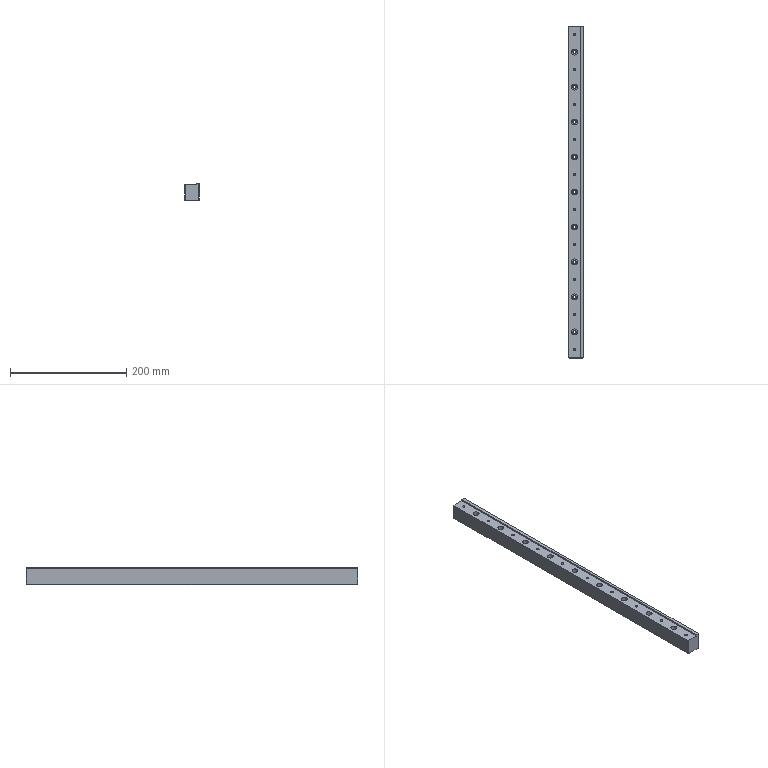Part | SolidWorks | features Chamfer 2, HoleWzd 2, Extrusion 1, ICE 1, LPattern 1 | 1 solid | 99 faces | box 25 x 570 x 30 mm | volume 386551 mm3 | cylinder 56 | plane 23 | cone 20 | commonest cylinder face diameters 4.2 x20 5.5 x18 10 x18